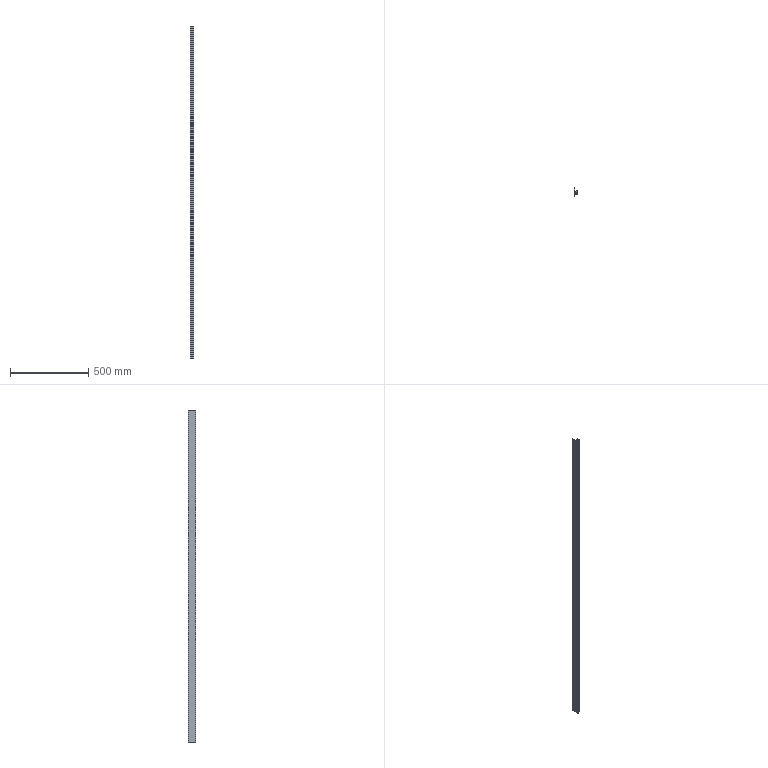Part | SolidWorks | features Extrusion 1 | 1 solid | 43 faces | box 25 x 50 x 2116 mm | volume 659198 mm3 | plane 35 | cylinder 8 | commonest cylinder face diameters 0.6 x8
STEP:
#1=CARTESIAN_POINT('',(1.5,0.,1058.));
#2=VERTEX_POINT('',#1);
#3=CARTESIAN_POINT('',(1.5,10.,1058.));
#4=VERTEX_POINT('',#3);
#5=CARTESIAN_POINT('',(1.5,0.,1058.));
#6=DIRECTION('',(0.,1.,0.));
#7=VECTOR('',#6,1000.);
#8=LINE('',#5,#7);
#9=EDGE_CURVE('',#2,#4,#8,.T.);
#10=ORIENTED_EDGE('',*,*,#9,.T.);
#11=CARTESIAN_POINT('',(4.,10.,1058.));
#12=VERTEX_POINT('',#11);
#13=CARTESIAN_POINT('',(1.5,10.,1058.));
#14=DIRECTION('',(1.,0.,0.));
#15=VECTOR('',#14,1000.);
#16=LINE('',#13,#15);
#17=EDGE_CURVE('',#4,#12,#16,.T.);
#18=ORIENTED_EDGE('',*,*,#17,.T.);
#19=CARTESIAN_POINT('',(4.,10.5,1058.));
#20=VERTEX_POINT('',#19);
#21=CARTESIAN_POINT('',(4.,10.,1058.));
#22=DIRECTION('',(0.,1.,0.));
#23=VECTOR('',#22,1000.);
#24=LINE('',#21,#23);
#25=EDGE_CURVE('',#12,#20,#24,.T.);
#26=ORIENTED_EDGE('',*,*,#25,.T.);
#27=CARTESIAN_POINT('',(8.9,10.5,1058.));
#28=VERTEX_POINT('',#27);
#29=CARTESIAN_POINT('',(4.,10.5,1058.));
#30=DIRECTION('',(1.,0.,0.));
#31=VECTOR('',#30,1000.);
#32=LINE('',#29,#31);
#33=EDGE_CURVE('',#20,#28,#32,.T.);
#34=ORIENTED_EDGE('',*,*,#33,.T.);
#35=CARTESIAN_POINT('',(8.9,12.2,1058.));
#36=VERTEX_POINT('',#35);
#37=CARTESIAN_POINT('',(8.9,10.5,1058.));
#38=DIRECTION('',(0.,1.,0.));
#39=VECTOR('',#38,1000.);
#40=LINE('',#37,#39);
#41=EDGE_CURVE('',#28,#36,#40,.T.);
#42=ORIENTED_EDGE('',*,*,#41,.T.);
#43=CARTESIAN_POINT('',(8.6,12.5,1058.));
#44=VERTEX_POINT('',#43);
#45=CARTESIAN_POINT('',(8.6,12.2,1058.));
#46=DIRECTION('',(0.,0.,1.));
#47=DIRECTION('',(1.,0.,0.));
#48=AXIS2_PLACEMENT_3D('',#45,#46,#47);
#49=CIRCLE('',#48,0.3);
#50=EDGE_CURVE('',#36,#44,#49,.T.);
#51=ORIENTED_EDGE('',*,*,#50,.T.);
#52=CARTESIAN_POINT('',(5.05,12.5,1058.));
#53=VERTEX_POINT('',#52);
#54=CARTESIAN_POINT('',(8.6,12.5,1058.));
#55=DIRECTION('',(-1.,0.,0.));
#56=VECTOR('',#55,1000.);
#57=LINE('',#54,#56);
#58=EDGE_CURVE('',#44,#53,#57,.T.);
#59=ORIENTED_EDGE('',*,*,#58,.T.);
#60=CARTESIAN_POINT('',(4.75,12.8,1058.));
#61=VERTEX_POINT('',#60);
#62=CARTESIAN_POINT('',(5.05,12.8,1058.));
#63=DIRECTION('',(0.,0.,-1.));
#64=DIRECTION('',(1.,0.,0.));
#65=AXIS2_PLACEMENT_3D('',#62,#63,#64);
#66=CIRCLE('',#65,0.3);
#67=EDGE_CURVE('',#53,#61,#66,.T.);
#68=ORIENTED_EDGE('',*,*,#67,.T.);
#69=CARTESIAN_POINT('',(4.75,16.153,1058.));
#70=VERTEX_POINT('',#69);
#71=CARTESIAN_POINT('',(4.75,12.8,1058.));
#72=DIRECTION('',(0.,1.,0.));
#73=VECTOR('',#72,1000.);
#74=LINE('',#71,#73);
#75=EDGE_CURVE('',#61,#70,#74,.T.);
#76=ORIENTED_EDGE('',*,*,#75,.T.);
#77=CARTESIAN_POINT('',(4.838,16.365,1058.));
#78=VERTEX_POINT('',#77);
#79=CARTESIAN_POINT('',(5.05,16.153,1058.));
#80=DIRECTION('',(0.,0.,-1.));
#81=DIRECTION('',(1.,0.,0.));
#82=AXIS2_PLACEMENT_3D('',#79,#80,#81);
#83=CIRCLE('',#82,0.3);
#84=EDGE_CURVE('',#70,#78,#83,.T.);
#85=ORIENTED_EDGE('',*,*,#84,.T.);
#86=CARTESIAN_POINT('',(8.785,20.312,1058.));
#87=VERTEX_POINT('',#86);
#88=CARTESIAN_POINT('',(4.838,16.365,1058.));
#89=DIRECTION('',(0.7071,0.7071,0.));
#90=VECTOR('',#89,1000.);
#91=LINE('',#88,#90);
#92=EDGE_CURVE('',#78,#87,#91,.T.);
#93=ORIENTED_EDGE('',*,*,#92,.T.);
#94=CARTESIAN_POINT('',(8.997,20.4,1058.));
#95=VERTEX_POINT('',#94);
#96=CARTESIAN_POINT('',(8.997,20.1,1058.));
#97=DIRECTION('',(0.,0.,-1.));
#98=DIRECTION('',(1.,0.,0.));
#99=AXIS2_PLACEMENT_3D('',#96,#97,#98);
#100=CIRCLE('',#99,0.3);
#101=EDGE_CURVE('',#87,#95,#100,.T.);
#102=ORIENTED_EDGE('',*,*,#101,.T.);
#103=CARTESIAN_POINT('',(17.003,20.4,1058.));
#104=VERTEX_POINT('',#103);
#105=CARTESIAN_POINT('',(8.997,20.4,1058.));
#106=DIRECTION('',(1.,0.,0.));
#107=VECTOR('',#106,1000.);
#108=LINE('',#105,#107);
#109=EDGE_CURVE('',#95,#104,#108,.T.);
#110=ORIENTED_EDGE('',*,*,#109,.T.);
#111=CARTESIAN_POINT('',(17.215,20.312,1058.));
#112=VERTEX_POINT('',#111);
#113=CARTESIAN_POINT('',(17.003,20.1,1058.));
#114=DIRECTION('',(0.,0.,-1.));
#115=DIRECTION('',(1.,0.,0.));
#116=AXIS2_PLACEMENT_3D('',#113,#114,#115);
#117=CIRCLE('',#116,0.3);
#118=EDGE_CURVE('',#104,#112,#117,.T.);
#119=ORIENTED_EDGE('',*,*,#118,.T.);
#120=CARTESIAN_POINT('',(21.162,16.365,1058.));
#121=VERTEX_POINT('',#120);
#122=CARTESIAN_POINT('',(17.215,20.312,1058.));
#123=DIRECTION('',(0.7071,-0.7071,0.));
#124=VECTOR('',#123,1000.);
#125=LINE('',#122,#124);
#126=EDGE_CURVE('',#112,#121,#125,.T.);
#127=ORIENTED_EDGE('',*,*,#126,.T.);
#128=CARTESIAN_POINT('',(21.25,16.153,1058.));
#129=VERTEX_POINT('',#128);
#130=CARTESIAN_POINT('',(20.95,16.153,1058.));
#131=DIRECTION('',(0.,0.,-1.));
#132=DIRECTION('',(1.,0.,0.));
#133=AXIS2_PLACEMENT_3D('',#130,#131,#132);
#134=CIRCLE('',#133,0.3);
#135=EDGE_CURVE('',#121,#129,#134,.T.);
#136=ORIENTED_EDGE('',*,*,#135,.T.);
#137=CARTESIAN_POINT('',(21.25,12.8,1058.));
#138=VERTEX_POINT('',#137);
#139=CARTESIAN_POINT('',(21.25,16.153,1058.));
#140=DIRECTION('',(0.,-1.,0.));
#141=VECTOR('',#140,1000.);
#142=LINE('',#139,#141);
#143=EDGE_CURVE('',#129,#138,#142,.T.);
#144=ORIENTED_EDGE('',*,*,#143,.T.);
#145=CARTESIAN_POINT('',(20.95,12.5,1058.));
#146=VERTEX_POINT('',#145);
#147=CARTESIAN_POINT('',(20.95,12.8,1058.));
#148=DIRECTION('',(0.,0.,-1.));
#149=DIRECTION('',(1.,0.,0.));
#150=AXIS2_PLACEMENT_3D('',#147,#148,#149);
#151=CIRCLE('',#150,0.3);
#152=EDGE_CURVE('',#138,#146,#151,.T.);
#153=ORIENTED_EDGE('',*,*,#152,.T.);
#154=CARTESIAN_POINT('',(17.4,12.5,1058.));
#155=VERTEX_POINT('',#154);
#156=CARTESIAN_POINT('',(20.95,12.5,1058.));
#157=DIRECTION('',(-1.,0.,0.));
#158=VECTOR('',#157,1000.);
#159=LINE('',#156,#158);
#160=EDGE_CURVE('',#146,#155,#159,.T.);
#161=ORIENTED_EDGE('',*,*,#160,.T.);
#162=CARTESIAN_POINT('',(17.1,12.2,1058.));
#163=VERTEX_POINT('',#162);
#164=CARTESIAN_POINT('',(17.4,12.2,1058.));
#165=DIRECTION('',(0.,0.,1.));
#166=DIRECTION('',(1.,0.,0.));
#167=AXIS2_PLACEMENT_3D('',#164,#165,#166);
#168=CIRCLE('',#167,0.3);
#169=EDGE_CURVE('',#155,#163,#168,.T.);
#170=ORIENTED_EDGE('',*,*,#169,.T.);
#171=CARTESIAN_POINT('',(17.1,10.5,1058.));
#172=VERTEX_POINT('',#171);
#173=CARTESIAN_POINT('',(17.1,12.2,1058.));
#174=DIRECTION('',(0.,-1.,0.));
#175=VECTOR('',#174,1000.);
#176=LINE('',#173,#175);
#177=EDGE_CURVE('',#163,#172,#176,.T.);
#178=ORIENTED_EDGE('',*,*,#177,.T.);
#179=CARTESIAN_POINT('',(22.,10.5,1058.));
#180=VERTEX_POINT('',#179);
#181=CARTESIAN_POINT('',(17.1,10.5,1058.));
#182=DIRECTION('',(1.,0.,0.));
#183=VECTOR('',#182,1000.);
#184=LINE('',#181,#183);
#185=EDGE_CURVE('',#172,#180,#184,.T.);
#186=ORIENTED_EDGE('',*,*,#185,.T.);
#187=CARTESIAN_POINT('',(22.,10.,1058.));
#188=VERTEX_POINT('',#187);
#189=CARTESIAN_POINT('',(22.,10.5,1058.));
#190=DIRECTION('',(0.,-1.,0.));
#191=VECTOR('',#190,1000.);
#192=LINE('',#189,#191);
#193=EDGE_CURVE('',#180,#188,#192,.T.);
#194=ORIENTED_EDGE('',*,*,#193,.T.);
#195=CARTESIAN_POINT('',(25.,10.,1058.));
#196=VERTEX_POINT('',#195);
#197=CARTESIAN_POINT('',(22.,10.,1058.));
#198=DIRECTION('',(1.,0.,0.));
#199=VECTOR('',#198,1000.);
#200=LINE('',#197,#199);
#201=EDGE_CURVE('',#188,#196,#200,.T.);
#202=ORIENTED_EDGE('',*,*,#201,.T.);
#203=CARTESIAN_POINT('',(25.,15.,1058.));
#204=VERTEX_POINT('',#203);
#205=CARTESIAN_POINT('',(25.,10.,1058.));
#206=DIRECTION('',(0.,1.,0.));
#207=VECTOR('',#206,1000.);
#208=LINE('',#205,#207);
#209=EDGE_CURVE('',#196,#204,#208,.T.);
#210=ORIENTED_EDGE('',*,*,#209,.T.);
#211=CARTESIAN_POINT('',(23.,15.,1058.));
#212=VERTEX_POINT('',#211);
#213=CARTESIAN_POINT('',(25.,15.,1058.));
#214=DIRECTION('',(-1.,0.,0.));
#215=VECTOR('',#214,1000.);
#216=LINE('',#213,#215);
#217=EDGE_CURVE('',#204,#212,#216,.T.);
#218=ORIENTED_EDGE('',*,*,#217,.T.);
#219=CARTESIAN_POINT('',(23.,29.246,1058.));
#220=VERTEX_POINT('',#219);
#221=CARTESIAN_POINT('',(23.,15.,1058.));
#222=DIRECTION('',(0.,1.,0.));
#223=VECTOR('',#222,1000.);
#224=LINE('',#221,#223);
#225=EDGE_CURVE('',#212,#220,#224,.T.);
#226=ORIENTED_EDGE('',*,*,#225,.T.);
#227=CARTESIAN_POINT('',(22.25,29.996,1058.));
#228=VERTEX_POINT('',#227);
#229=CARTESIAN_POINT('',(23.,29.246,1058.));
#230=DIRECTION('',(-0.7071,0.7071,0.));
#231=VECTOR('',#230,1000.);
#232=LINE('',#229,#231);
#233=EDGE_CURVE('',#220,#228,#232,.T.);
#234=ORIENTED_EDGE('',*,*,#233,.T.);
#235=CARTESIAN_POINT('',(4.,30.,1058.));
#236=VERTEX_POINT('',#235);
#237=CARTESIAN_POINT('',(22.25,29.996,1058.));
#238=DIRECTION('',(-1.,0.0002341,0.));
#239=VECTOR('',#238,1000.);
#240=LINE('',#237,#239);
#241=EDGE_CURVE('',#228,#236,#240,.T.);
#242=ORIENTED_EDGE('',*,*,#241,.T.);
#243=CARTESIAN_POINT('',(4.,34.998,1058.));
#244=VERTEX_POINT('',#243);
#245=CARTESIAN_POINT('',(4.,30.,1058.));
#246=DIRECTION('',(0.,1.,0.));
#247=VECTOR('',#246,1000.);
#248=LINE('',#245,#247);
#249=EDGE_CURVE('',#236,#244,#248,.T.);
#250=ORIENTED_EDGE('',*,*,#249,.T.);
#251=CARTESIAN_POINT('',(3.,34.998,1058.));
#252=VERTEX_POINT('',#251);
#253=CARTESIAN_POINT('',(4.,34.998,1058.));
#254=DIRECTION('',(-1.,0.,0.));
#255=VECTOR('',#254,1000.);
#256=LINE('',#253,#255);
#257=EDGE_CURVE('',#244,#252,#256,.T.);
#258=ORIENTED_EDGE('',*,*,#257,.T.);
#259=CARTESIAN_POINT('',(3.,43.,1058.));
#260=VERTEX_POINT('',#259);
#261=CARTESIAN_POINT('',(3.,34.998,1058.));
#262=DIRECTION('',(0.,1.,0.));
#263=VECTOR('',#262,1000.);
#264=LINE('',#261,#263);
#265=EDGE_CURVE('',#252,#260,#264,.T.);
#266=ORIENTED_EDGE('',*,*,#265,.T.);
#267=CARTESIAN_POINT('',(4.,43.,1058.));
#268=VERTEX_POINT('',#267);
#269=CARTESIAN_POINT('',(3.,43.,1058.));
#270=DIRECTION('',(1.,0.,0.));
#271=VECTOR('',#270,1000.);
#272=LINE('',#269,#271);
#273=EDGE_CURVE('',#260,#268,#272,.T.);
#274=ORIENTED_EDGE('',*,*,#273,.T.);
#275=CARTESIAN_POINT('',(4.,50.,1058.));
#276=VERTEX_POINT('',#275);
#277=CARTESIAN_POINT('',(4.,43.,1058.));
#278=DIRECTION('',(0.,1.,0.));
#279=VECTOR('',#278,1000.);
#280=LINE('',#277,#279);
#281=EDGE_CURVE('',#268,#276,#280,.T.);
#282=ORIENTED_EDGE('',*,*,#281,.T.);
#283=CARTESIAN_POINT('',(0.,50.,1058.));
#284=VERTEX_POINT('',#283);
#285=CARTESIAN_POINT('',(4.,50.,1058.));
#286=DIRECTION('',(-1.,0.,0.));
#287=VECTOR('',#286,1000.);
#288=LINE('',#285,#287);
#289=EDGE_CURVE('',#276,#284,#288,.T.);
#290=ORIENTED_EDGE('',*,*,#289,.T.);
#291=CARTESIAN_POINT('',(0.,0.,1058.));
#292=VERTEX_POINT('',#291);
#293=CARTESIAN_POINT('',(0.,50.,1058.));
#294=DIRECTION('',(0.,-1.,0.));
#295=VECTOR('',#294,1000.);
#296=LINE('',#293,#295);
#297=EDGE_CURVE('',#284,#292,#296,.T.);
#298=ORIENTED_EDGE('',*,*,#297,.T.);
#299=CARTESIAN_POINT('',(0.,0.,1058.));
#300=DIRECTION('',(1.,0.,0.));
#301=VECTOR('',#300,1000.);
#302=LINE('',#299,#301);
#303=EDGE_CURVE('',#292,#2,#302,.T.);
#304=ORIENTED_EDGE('',*,*,#303,.T.);
#305=EDGE_LOOP('',(#10,#18,#26,#34,#42,#51,#59,#68,#76,#85,#93,#102,#110,#119,#127,#136,#144,#153,#161,#170,#178,#186,#194,#202,#210,#218,#226,#234,#242,#250,#258,#266,#274,#282,#290,#298,#304));
#306=FACE_OUTER_BOUND('',#305,.T.);
#307=CARTESIAN_POINT('',(21.,28.,1058.));
#308=VERTEX_POINT('',#307);
#309=CARTESIAN_POINT('',(2.,28.,1058.));
#310=VERTEX_POINT('',#309);
#311=CARTESIAN_POINT('',(2.,28.,1058.));
#312=DIRECTION('',(-1.,0.,0.));
#313=VECTOR('',#312,1000.);
#314=LINE('',#311,#313);
#315=EDGE_CURVE('',#308,#310,#314,.T.);
#316=ORIENTED_EDGE('',*,*,#315,.F.);
#317=CARTESIAN_POINT('',(21.,22.4,1058.));
#318=VERTEX_POINT('',#317);
#319=CARTESIAN_POINT('',(21.,28.,1058.));
#320=DIRECTION('',(0.,1.,0.));
#321=VECTOR('',#320,1000.);
#322=LINE('',#319,#321);
#323=EDGE_CURVE('',#318,#308,#322,.T.);
#324=ORIENTED_EDGE('',*,*,#323,.F.);
#325=CARTESIAN_POINT('',(2.,22.4,1058.));
#326=VERTEX_POINT('',#325);
#327=CARTESIAN_POINT('',(21.,22.4,1058.));
#328=DIRECTION('',(1.,0.,0.));
#329=VECTOR('',#328,1000.);
#330=LINE('',#327,#329);
#331=EDGE_CURVE('',#326,#318,#330,.T.);
#332=ORIENTED_EDGE('',*,*,#331,.F.);
#333=CARTESIAN_POINT('',(2.,22.4,1058.));
#334=DIRECTION('',(0.,-1.,0.));
#335=VECTOR('',#334,1000.);
#336=LINE('',#333,#335);
#337=EDGE_CURVE('',#310,#326,#336,.T.);
#338=ORIENTED_EDGE('',*,*,#337,.F.);
#339=EDGE_LOOP('',(#316,#324,#332,#338));
#340=FACE_BOUND('',#339,.T.);
#341=CARTESIAN_POINT('',(8.6,12.2,1058.));
#342=DIRECTION('',(0.,0.,1.));
#343=DIRECTION('',(1.,0.,0.));
#344=AXIS2_PLACEMENT_3D('',#341,#342,#343);
#345=PLANE('',#344);
#346=ADVANCED_FACE('',(#306,#340),#345,.T.);
#347=CARTESIAN_POINT('',(1.5,0.,-1058.));
#348=VERTEX_POINT('',#347);
#349=CARTESIAN_POINT('',(1.5,10.,-1058.));
#350=VERTEX_POINT('',#349);
#351=CARTESIAN_POINT('',(1.5,0.,-1058.));
#352=DIRECTION('',(0.,1.,0.));
#353=VECTOR('',#352,1000.);
#354=LINE('',#351,#353);
#355=EDGE_CURVE('',#348,#350,#354,.T.);
#356=ORIENTED_EDGE('',*,*,#355,.F.);
#357=CARTESIAN_POINT('',(0.,0.,-1058.));
#358=VERTEX_POINT('',#357);
#359=CARTESIAN_POINT('',(0.,0.,-1058.));
#360=DIRECTION('',(1.,0.,0.));
#361=VECTOR('',#360,1000.);
#362=LINE('',#359,#361);
#363=EDGE_CURVE('',#358,#348,#362,.T.);
#364=ORIENTED_EDGE('',*,*,#363,.F.);
#365=CARTESIAN_POINT('',(0.,50.,-1058.));
#366=VERTEX_POINT('',#365);
#367=CARTESIAN_POINT('',(0.,50.,-1058.));
#368=DIRECTION('',(0.,-1.,0.));
#369=VECTOR('',#368,1000.);
#370=LINE('',#367,#369);
#371=EDGE_CURVE('',#366,#358,#370,.T.);
#372=ORIENTED_EDGE('',*,*,#371,.F.);
#373=CARTESIAN_POINT('',(4.,50.,-1058.));
#374=VERTEX_POINT('',#373);
#375=CARTESIAN_POINT('',(4.,50.,-1058.));
#376=DIRECTION('',(-1.,0.,0.));
#377=VECTOR('',#376,1000.);
#378=LINE('',#375,#377);
#379=EDGE_CURVE('',#374,#366,#378,.T.);
#380=ORIENTED_EDGE('',*,*,#379,.F.);
#381=CARTESIAN_POINT('',(4.,43.,-1058.));
#382=VERTEX_POINT('',#381);
#383=CARTESIAN_POINT('',(4.,43.,-1058.));
#384=DIRECTION('',(0.,1.,0.));
#385=VECTOR('',#384,1000.);
#386=LINE('',#383,#385);
#387=EDGE_CURVE('',#382,#374,#386,.T.);
#388=ORIENTED_EDGE('',*,*,#387,.F.);
#389=CARTESIAN_POINT('',(3.,43.,-1058.));
#390=VERTEX_POINT('',#389);
#391=CARTESIAN_POINT('',(3.,43.,-1058.));
#392=DIRECTION('',(1.,0.,0.));
#393=VECTOR('',#392,1000.);
#394=LINE('',#391,#393);
#395=EDGE_CURVE('',#390,#382,#394,.T.);
#396=ORIENTED_EDGE('',*,*,#395,.F.);
#397=CARTESIAN_POINT('',(3.,34.998,-1058.));
#398=VERTEX_POINT('',#397);
#399=CARTESIAN_POINT('',(3.,34.998,-1058.));
#400=DIRECTION('',(0.,1.,0.));
#401=VECTOR('',#400,1000.);
#402=LINE('',#399,#401);
#403=EDGE_CURVE('',#398,#390,#402,.T.);
#404=ORIENTED_EDGE('',*,*,#403,.F.);
#405=CARTESIAN_POINT('',(4.,34.998,-1058.));
#406=VERTEX_POINT('',#405);
#407=CARTESIAN_POINT('',(4.,34.998,-1058.));
#408=DIRECTION('',(-1.,0.,0.));
#409=VECTOR('',#408,1000.);
#410=LINE('',#407,#409);
#411=EDGE_CURVE('',#406,#398,#410,.T.);
#412=ORIENTED_EDGE('',*,*,#411,.F.);
#413=CARTESIAN_POINT('',(4.,30.,-1058.));
#414=VERTEX_POINT('',#413);
#415=CARTESIAN_POINT('',(4.,30.,-1058.));
#416=DIRECTION('',(0.,1.,0.));
#417=VECTOR('',#416,1000.);
#418=LINE('',#415,#417);
#419=EDGE_CURVE('',#414,#406,#418,.T.);
#420=ORIENTED_EDGE('',*,*,#419,.F.);
#421=CARTESIAN_POINT('',(22.25,29.996,-1058.));
#422=VERTEX_POINT('',#421);
#423=CARTESIAN_POINT('',(22.25,29.996,-1058.));
#424=DIRECTION('',(-1.,0.0002341,0.));
#425=VECTOR('',#424,1000.);
#426=LINE('',#423,#425);
#427=EDGE_CURVE('',#422,#414,#426,.T.);
#428=ORIENTED_EDGE('',*,*,#427,.F.);
#429=CARTESIAN_POINT('',(23.,29.246,-1058.));
#430=VERTEX_POINT('',#429);
#431=CARTESIAN_POINT('',(23.,29.246,-1058.));
#432=DIRECTION('',(-0.7071,0.7071,0.));
#433=VECTOR('',#432,1000.);
#434=LINE('',#431,#433);
#435=EDGE_CURVE('',#430,#422,#434,.T.);
#436=ORIENTED_EDGE('',*,*,#435,.F.);
#437=CARTESIAN_POINT('',(23.,15.,-1058.));
#438=VERTEX_POINT('',#437);
#439=CARTESIAN_POINT('',(23.,15.,-1058.));
#440=DIRECTION('',(0.,1.,0.));
#441=VECTOR('',#440,1000.);
#442=LINE('',#439,#441);
#443=EDGE_CURVE('',#438,#430,#442,.T.);
#444=ORIENTED_EDGE('',*,*,#443,.F.);
#445=CARTESIAN_POINT('',(25.,15.,-1058.));
#446=VERTEX_POINT('',#445);
#447=CARTESIAN_POINT('',(25.,15.,-1058.));
#448=DIRECTION('',(-1.,0.,0.));
#449=VECTOR('',#448,1000.);
#450=LINE('',#447,#449);
#451=EDGE_CURVE('',#446,#438,#450,.T.);
#452=ORIENTED_EDGE('',*,*,#451,.F.);
#453=CARTESIAN_POINT('',(25.,10.,-1058.));
#454=VERTEX_POINT('',#453);
#455=CARTESIAN_POINT('',(25.,10.,-1058.));
#456=DIRECTION('',(0.,1.,0.));
#457=VECTOR('',#456,1000.);
#458=LINE('',#455,#457);
#459=EDGE_CURVE('',#454,#446,#458,.T.);
#460=ORIENTED_EDGE('',*,*,#459,.F.);
#461=CARTESIAN_POINT('',(22.,10.,-1058.));
#462=VERTEX_POINT('',#461);
#463=CARTESIAN_POINT('',(22.,10.,-1058.));
#464=DIRECTION('',(1.,0.,0.));
#465=VECTOR('',#464,1000.);
#466=LINE('',#463,#465);
#467=EDGE_CURVE('',#462,#454,#466,.T.);
#468=ORIENTED_EDGE('',*,*,#467,.F.);
#469=CARTESIAN_POINT('',(22.,10.5,-1058.));
#470=VERTEX_POINT('',#469);
#471=CARTESIAN_POINT('',(22.,10.5,-1058.));
#472=DIRECTION('',(0.,-1.,0.));
#473=VECTOR('',#472,1000.);
#474=LINE('',#471,#473);
#475=EDGE_CURVE('',#470,#462,#474,.T.);
#476=ORIENTED_EDGE('',*,*,#475,.F.);
#477=CARTESIAN_POINT('',(17.1,10.5,-1058.));
#478=VERTEX_POINT('',#477);
#479=CARTESIAN_POINT('',(17.1,10.5,-1058.));
#480=DIRECTION('',(1.,0.,0.));
#481=VECTOR('',#480,1000.);
#482=LINE('',#479,#481);
#483=EDGE_CURVE('',#478,#470,#482,.T.);
#484=ORIENTED_EDGE('',*,*,#483,.F.);
#485=CARTESIAN_POINT('',(17.1,12.2,-1058.));
#486=VERTEX_POINT('',#485);
#487=CARTESIAN_POINT('',(17.1,12.2,-1058.));
#488=DIRECTION('',(0.,-1.,0.));
#489=VECTOR('',#488,1000.);
#490=LINE('',#487,#489);
#491=EDGE_CURVE('',#486,#478,#490,.T.);
#492=ORIENTED_EDGE('',*,*,#491,.F.);
#493=CARTESIAN_POINT('',(17.4,12.5,-1058.));
#494=VERTEX_POINT('',#493);
#495=CARTESIAN_POINT('',(17.4,12.2,-1058.));
#496=DIRECTION('',(0.,0.,1.));
#497=DIRECTION('',(1.,0.,0.));
#498=AXIS2_PLACEMENT_3D('',#495,#496,#497);
#499=CIRCLE('',#498,0.3);
#500=EDGE_CURVE('',#494,#486,#499,.T.);
#501=ORIENTED_EDGE('',*,*,#500,.F.);
#502=CARTESIAN_POINT('',(20.95,12.5,-1058.));
#503=VERTEX_POINT('',#502);
#504=CARTESIAN_POINT('',(20.95,12.5,-1058.));
#505=DIRECTION('',(-1.,0.,0.));
#506=VECTOR('',#505,1000.);
#507=LINE('',#504,#506);
#508=EDGE_CURVE('',#503,#494,#507,.T.);
#509=ORIENTED_EDGE('',*,*,#508,.F.);
#510=CARTESIAN_POINT('',(21.25,12.8,-1058.));
#511=VERTEX_POINT('',#510);
#512=CARTESIAN_POINT('',(20.95,12.8,-1058.));
#513=DIRECTION('',(0.,0.,-1.));
#514=DIRECTION('',(1.,0.,0.));
#515=AXIS2_PLACEMENT_3D('',#512,#513,#514);
#516=CIRCLE('',#515,0.3);
#517=EDGE_CURVE('',#511,#503,#516,.T.);
#518=ORIENTED_EDGE('',*,*,#517,.F.);
#519=CARTESIAN_POINT('',(21.25,16.153,-1058.));
#520=VERTEX_POINT('',#519);
#521=CARTESIAN_POINT('',(21.25,16.153,-1058.));
#522=DIRECTION('',(0.,-1.,0.));
#523=VECTOR('',#522,1000.);
#524=LINE('',#521,#523);
#525=EDGE_CURVE('',#520,#511,#524,.T.);
#526=ORIENTED_EDGE('',*,*,#525,.F.);
#527=CARTESIAN_POINT('',(21.162,16.365,-1058.));
#528=VERTEX_POINT('',#527);
#529=CARTESIAN_POINT('',(20.95,16.153,-1058.));
#530=DIRECTION('',(0.,0.,-1.));
#531=DIRECTION('',(1.,0.,0.));
#532=AXIS2_PLACEMENT_3D('',#529,#530,#531);
#533=CIRCLE('',#532,0.3);
#534=EDGE_CURVE('',#528,#520,#533,.T.);
#535=ORIENTED_EDGE('',*,*,#534,.F.);
#536=CARTESIAN_POINT('',(17.215,20.312,-1058.));
#537=VERTEX_POINT('',#536);
#538=CARTESIAN_POINT('',(17.215,20.312,-1058.));
#539=DIRECTION('',(0.7071,-0.7071,0.));
#540=VECTOR('',#539,1000.);
#541=LINE('',#538,#540);
#542=EDGE_CURVE('',#537,#528,#541,.T.);
#543=ORIENTED_EDGE('',*,*,#542,.F.);
#544=CARTESIAN_POINT('',(17.003,20.4,-1058.));
#545=VERTEX_POINT('',#544);
#546=CARTESIAN_POINT('',(17.003,20.1,-1058.));
#547=DIRECTION('',(0.,0.,-1.));
#548=DIRECTION('',(1.,0.,0.));
#549=AXIS2_PLACEMENT_3D('',#546,#547,#548);
#550=CIRCLE('',#549,0.3);
#551=EDGE_CURVE('',#545,#537,#550,.T.);
#552=ORIENTED_EDGE('',*,*,#551,.F.);
#553=CARTESIAN_POINT('',(8.997,20.4,-1058.));
#554=VERTEX_POINT('',#553);
#555=CARTESIAN_POINT('',(8.997,20.4,-1058.));
#556=DIRECTION('',(1.,0.,0.));
#557=VECTOR('',#556,1000.);
#558=LINE('',#555,#557);
#559=EDGE_CURVE('',#554,#545,#558,.T.);
#560=ORIENTED_EDGE('',*,*,#559,.F.);
#561=CARTESIAN_POINT('',(8.785,20.312,-1058.));
#562=VERTEX_POINT('',#561);
#563=CARTESIAN_POINT('',(8.997,20.1,-1058.));
#564=DIRECTION('',(0.,0.,-1.));
#565=DIRECTION('',(1.,0.,0.));
#566=AXIS2_PLACEMENT_3D('',#563,#564,#565);
#567=CIRCLE('',#566,0.3);
#568=EDGE_CURVE('',#562,#554,#567,.T.);
#569=ORIENTED_EDGE('',*,*,#568,.F.);
#570=CARTESIAN_POINT('',(4.838,16.365,-1058.));
#571=VERTEX_POINT('',#570);
#572=CARTESIAN_POINT('',(4.838,16.365,-1058.));
#573=DIRECTION('',(0.7071,0.7071,0.));
#574=VECTOR('',#573,1000.);
#575=LINE('',#572,#574);
#576=EDGE_CURVE('',#571,#562,#575,.T.);
#577=ORIENTED_EDGE('',*,*,#576,.F.);
#578=CARTESIAN_POINT('',(4.75,16.153,-1058.));
#579=VERTEX_POINT('',#578);
#580=CARTESIAN_POINT('',(5.05,16.153,-1058.));
#581=DIRECTION('',(0.,0.,-1.));
#582=DIRECTION('',(1.,0.,0.));
#583=AXIS2_PLACEMENT_3D('',#580,#581,#582);
#584=CIRCLE('',#583,0.3);
#585=EDGE_CURVE('',#579,#571,#584,.T.);
#586=ORIENTED_EDGE('',*,*,#585,.F.);
#587=CARTESIAN_POINT('',(4.75,12.8,-1058.));
#588=VERTEX_POINT('',#587);
#589=CARTESIAN_POINT('',(4.75,12.8,-1058.));
#590=DIRECTION('',(0.,1.,0.));
#591=VECTOR('',#590,1000.);
#592=LINE('',#589,#591);
#593=EDGE_CURVE('',#588,#579,#592,.T.);
#594=ORIENTED_EDGE('',*,*,#593,.F.);
#595=CARTESIAN_POINT('',(5.05,12.5,-1058.));
#596=VERTEX_POINT('',#595);
#597=CARTESIAN_POINT('',(5.05,12.8,-1058.));
#598=DIRECTION('',(0.,0.,-1.));
#599=DIRECTION('',(1.,0.,0.));
#600=AXIS2_PLACEMENT_3D('',#597,#598,#599);
#601=CIRCLE('',#600,0.3);
#602=EDGE_CURVE('',#596,#588,#601,.T.);
#603=ORIENTED_EDGE('',*,*,#602,.F.);
#604=CARTESIAN_POINT('',(8.6,12.5,-1058.));
#605=VERTEX_POINT('',#604);
#606=CARTESIAN_POINT('',(8.6,12.5,-1058.));
#607=DIRECTION('',(-1.,0.,0.));
#608=VECTOR('',#607,1000.);
#609=LINE('',#606,#608);
#610=EDGE_CURVE('',#605,#596,#609,.T.);
#611=ORIENTED_EDGE('',*,*,#610,.F.);
#612=CARTESIAN_POINT('',(8.9,12.2,-1058.));
#613=VERTEX_POINT('',#612);
#614=CARTESIAN_POINT('',(8.6,12.2,-1058.));
#615=DIRECTION('',(0.,0.,1.));
#616=DIRECTION('',(1.,0.,0.));
#617=AXIS2_PLACEMENT_3D('',#614,#615,#616);
#618=CIRCLE('',#617,0.3);
#619=EDGE_CURVE('',#613,#605,#618,.T.);
#620=ORIENTED_EDGE('',*,*,#619,.F.);
#621=CARTESIAN_POINT('',(8.9,10.5,-1058.));
#622=VERTEX_POINT('',#621);
#623=CARTESIAN_POINT('',(8.9,10.5,-1058.));
#624=DIRECTION('',(0.,1.,0.));
#625=VECTOR('',#624,1000.);
#626=LINE('',#623,#625);
#627=EDGE_CURVE('',#622,#613,#626,.T.);
#628=ORIENTED_EDGE('',*,*,#627,.F.);
#629=CARTESIAN_POINT('',(4.,10.5,-1058.));
#630=VERTEX_POINT('',#629);
#631=CARTESIAN_POINT('',(4.,10.5,-1058.));
#632=DIRECTION('',(1.,0.,0.));
#633=VECTOR('',#632,1000.);
#634=LINE('',#631,#633);
#635=EDGE_CURVE('',#630,#622,#634,.T.);
#636=ORIENTED_EDGE('',*,*,#635,.F.);
#637=CARTESIAN_POINT('',(4.,10.,-1058.));
#638=VERTEX_POINT('',#637);
#639=CARTESIAN_POINT('',(4.,10.,-1058.));
#640=DIRECTION('',(0.,1.,0.));
#641=VECTOR('',#640,1000.);
#642=LINE('',#639,#641);
#643=EDGE_CURVE('',#638,#630,#642,.T.);
#644=ORIENTED_EDGE('',*,*,#643,.F.);
#645=CARTESIAN_POINT('',(1.5,10.,-1058.));
#646=DIRECTION('',(1.,0.,0.));
#647=VECTOR('',#646,1000.);
#648=LINE('',#645,#647);
#649=EDGE_CURVE('',#350,#638,#648,.T.);
#650=ORIENTED_EDGE('',*,*,#649,.F.);
#651=EDGE_LOOP('',(#356,#364,#372,#380,#388,#396,#404,#412,#420,#428,#436,#444,#452,#460,#468,#476,#484,#492,#501,#509,#518,#526,#535,#543,#552,#560,#569,#577,#586,#594,#603,#611,#620,#628,#636,#644,#650));
#652=FACE_OUTER_BOUND('',#651,.T.);
#653=CARTESIAN_POINT('',(21.,22.4,-1058.));
#654=VERTEX_POINT('',#653);
#655=CARTESIAN_POINT('',(21.,28.,-1058.));
#656=VERTEX_POINT('',#655);
#657=CARTESIAN_POINT('',(21.,28.,-1058.));
#658=DIRECTION('',(0.,1.,0.));
#659=VECTOR('',#658,1000.);
#660=LINE('',#657,#659);
#661=EDGE_CURVE('',#654,#656,#660,.T.);
#662=ORIENTED_EDGE('',*,*,#661,.T.);
#663=CARTESIAN_POINT('',(2.,28.,-1058.));
#664=VERTEX_POINT('',#663);
#665=CARTESIAN_POINT('',(2.,28.,-1058.));
#666=DIRECTION('',(-1.,0.,0.));
#667=VECTOR('',#666,1000.);
#668=LINE('',#665,#667);
#669=EDGE_CURVE('',#656,#664,#668,.T.);
#670=ORIENTED_EDGE('',*,*,#669,.T.);
#671=CARTESIAN_POINT('',(2.,22.4,-1058.));
#672=VERTEX_POINT('',#671);
#673=CARTESIAN_POINT('',(2.,22.4,-1058.));
#674=DIRECTION('',(0.,-1.,0.));
#675=VECTOR('',#674,1000.);
#676=LINE('',#673,#675);
#677=EDGE_CURVE('',#664,#672,#676,.T.);
#678=ORIENTED_EDGE('',*,*,#677,.T.);
#679=CARTESIAN_POINT('',(21.,22.4,-1058.));
#680=DIRECTION('',(1.,0.,0.));
#681=VECTOR('',#680,1000.);
#682=LINE('',#679,#681);
#683=EDGE_CURVE('',#672,#654,#682,.T.);
#684=ORIENTED_EDGE('',*,*,#683,.T.);
#685=EDGE_LOOP('',(#662,#670,#678,#684));
#686=FACE_BOUND('',#685,.T.);
#687=CARTESIAN_POINT('',(8.6,12.2,-1058.));
#688=DIRECTION('',(0.,0.,1.));
#689=DIRECTION('',(1.,0.,0.));
#690=AXIS2_PLACEMENT_3D('',#687,#688,#689);
#691=PLANE('',#690);
#692=ADVANCED_FACE('',(#652,#686),#691,.F.);
#693=ORIENTED_EDGE('',*,*,#355,.T.);
#694=CARTESIAN_POINT('',(1.5,10.,1058.));
#695=DIRECTION('',(0.,0.,-1.));
#696=VECTOR('',#695,1000.);
#697=LINE('',#694,#696);
#698=EDGE_CURVE('',#4,#350,#697,.T.);
#699=ORIENTED_EDGE('',*,*,#698,.F.);
#700=ORIENTED_EDGE('',*,*,#9,.F.);
#701=CARTESIAN_POINT('',(1.5,0.,1058.));
#702=DIRECTION('',(0.,0.,-1.));
#703=VECTOR('',#702,1000.);
#704=LINE('',#701,#703);
#705=EDGE_CURVE('',#2,#348,#704,.T.);
#706=ORIENTED_EDGE('',*,*,#705,.T.);
#707=EDGE_LOOP('',(#693,#699,#700,#706));
#708=FACE_OUTER_BOUND('',#707,.T.);
#709=CARTESIAN_POINT('',(1.5,0.,1058.));
#710=DIRECTION('',(-1.,0.,0.));
#711=DIRECTION('',(0.,0.,1.));
#712=AXIS2_PLACEMENT_3D('',#709,#710,#711);
#713=PLANE('',#712);
#714=ADVANCED_FACE('',(#708),#713,.F.);
#715=ORIENTED_EDGE('',*,*,#649,.T.);
#716=CARTESIAN_POINT('',(4.,10.,1058.));
#717=DIRECTION('',(0.,0.,-1.));
#718=VECTOR('',#717,1000.);
#719=LINE('',#716,#718);
#720=EDGE_CURVE('',#12,#638,#719,.T.);
#721=ORIENTED_EDGE('',*,*,#720,.F.);
#722=ORIENTED_EDGE('',*,*,#17,.F.);
#723=ORIENTED_EDGE('',*,*,#698,.T.);
#724=EDGE_LOOP('',(#715,#721,#722,#723));
#725=FACE_OUTER_BOUND('',#724,.T.);
#726=CARTESIAN_POINT('',(1.5,10.,1058.));
#727=DIRECTION('',(0.,1.,0.));
#728=DIRECTION('',(0.,0.,1.));
#729=AXIS2_PLACEMENT_3D('',#726,#727,#728);
#730=PLANE('',#729);
#731=ADVANCED_FACE('',(#725),#730,.F.);
#732=ORIENTED_EDGE('',*,*,#643,.T.);
#733=CARTESIAN_POINT('',(4.,10.5,1058.));
#734=DIRECTION('',(0.,0.,-1.));
#735=VECTOR('',#734,1000.);
#736=LINE('',#733,#735);
#737=EDGE_CURVE('',#20,#630,#736,.T.);
#738=ORIENTED_EDGE('',*,*,#737,.F.);
#739=ORIENTED_EDGE('',*,*,#25,.F.);
#740=ORIENTED_EDGE('',*,*,#720,.T.);
#741=EDGE_LOOP('',(#732,#738,#739,#740));
#742=FACE_OUTER_BOUND('',#741,.T.);
#743=CARTESIAN_POINT('',(4.,10.,1058.));
#744=DIRECTION('',(-1.,0.,0.));
#745=DIRECTION('',(0.,0.,1.));
#746=AXIS2_PLACEMENT_3D('',#743,#744,#745);
#747=PLANE('',#746);
#748=ADVANCED_FACE('',(#742),#747,.F.);
#749=ORIENTED_EDGE('',*,*,#635,.T.);
#750=CARTESIAN_POINT('',(8.9,10.5,1058.));
#751=DIRECTION('',(0.,0.,-1.));
#752=VECTOR('',#751,1000.);
#753=LINE('',#750,#752);
#754=EDGE_CURVE('',#28,#622,#753,.T.);
#755=ORIENTED_EDGE('',*,*,#754,.F.);
#756=ORIENTED_EDGE('',*,*,#33,.F.);
#757=ORIENTED_EDGE('',*,*,#737,.T.);
#758=EDGE_LOOP('',(#749,#755,#756,#757));
#759=FACE_OUTER_BOUND('',#758,.T.);
#760=CARTESIAN_POINT('',(4.,10.5,1058.));
#761=DIRECTION('',(0.,1.,0.));
#762=DIRECTION('',(0.,0.,1.));
#763=AXIS2_PLACEMENT_3D('',#760,#761,#762);
#764=PLANE('',#763);
#765=ADVANCED_FACE('',(#759),#764,.F.);
#766=ORIENTED_EDGE('',*,*,#627,.T.);
#767=CARTESIAN_POINT('',(8.9,12.2,1058.));
#768=DIRECTION('',(0.,0.,-1.));
#769=VECTOR('',#768,1000.);
#770=LINE('',#767,#769);
#771=EDGE_CURVE('',#36,#613,#770,.T.);
#772=ORIENTED_EDGE('',*,*,#771,.F.);
#773=ORIENTED_EDGE('',*,*,#41,.F.);
#774=ORIENTED_EDGE('',*,*,#754,.T.);
#775=EDGE_LOOP('',(#766,#772,#773,#774));
#776=FACE_OUTER_BOUND('',#775,.T.);
#777=CARTESIAN_POINT('',(8.9,10.5,1058.));
#778=DIRECTION('',(-1.,0.,0.));
#779=DIRECTION('',(0.,0.,1.));
#780=AXIS2_PLACEMENT_3D('',#777,#778,#779);
#781=PLANE('',#780);
#782=ADVANCED_FACE('',(#776),#781,.F.);
#783=ORIENTED_EDGE('',*,*,#619,.T.);
#784=CARTESIAN_POINT('',(8.6,12.5,1058.));
#785=DIRECTION('',(0.,0.,-1.));
#786=VECTOR('',#785,1000.);
#787=LINE('',#784,#786);
#788=EDGE_CURVE('',#44,#605,#787,.T.);
#789=ORIENTED_EDGE('',*,*,#788,.F.);
#790=ORIENTED_EDGE('',*,*,#50,.F.);
#791=ORIENTED_EDGE('',*,*,#771,.T.);
#792=EDGE_LOOP('',(#783,#789,#790,#791));
#793=FACE_OUTER_BOUND('',#792,.T.);
#794=CARTESIAN_POINT('',(8.6,12.2,1058.));
#795=DIRECTION('',(0.,0.,-1.));
#796=DIRECTION('',(-1.,0.,0.));
#797=AXIS2_PLACEMENT_3D('',#794,#795,#796);
#798=CYLINDRICAL_SURFACE('',#797,0.3);
#799=ADVANCED_FACE('',(#793),#798,.T.);
#800=ORIENTED_EDGE('',*,*,#610,.T.);
#801=CARTESIAN_POINT('',(5.05,12.5,1058.));
#802=DIRECTION('',(0.,0.,-1.));
#803=VECTOR('',#802,1000.);
#804=LINE('',#801,#803);
#805=EDGE_CURVE('',#53,#596,#804,.T.);
#806=ORIENTED_EDGE('',*,*,#805,.F.);
#807=ORIENTED_EDGE('',*,*,#58,.F.);
#808=ORIENTED_EDGE('',*,*,#788,.T.);
#809=EDGE_LOOP('',(#800,#806,#807,#808));
#810=FACE_OUTER_BOUND('',#809,.T.);
#811=CARTESIAN_POINT('',(8.6,12.5,1058.));
#812=DIRECTION('',(0.,-1.,0.));
#813=DIRECTION('',(0.,0.,-1.));
#814=AXIS2_PLACEMENT_3D('',#811,#812,#813);
#815=PLANE('',#814);
#816=ADVANCED_FACE('',(#810),#815,.F.);
#817=ORIENTED_EDGE('',*,*,#602,.T.);
#818=CARTESIAN_POINT('',(4.75,12.8,1058.));
#819=DIRECTION('',(0.,0.,-1.));
#820=VECTOR('',#819,1000.);
#821=LINE('',#818,#820);
#822=EDGE_CURVE('',#61,#588,#821,.T.);
#823=ORIENTED_EDGE('',*,*,#822,.F.);
#824=ORIENTED_EDGE('',*,*,#67,.F.);
#825=ORIENTED_EDGE('',*,*,#805,.T.);
#826=EDGE_LOOP('',(#817,#823,#824,#825));
#827=FACE_OUTER_BOUND('',#826,.T.);
#828=CARTESIAN_POINT('',(5.05,12.8,1058.));
#829=DIRECTION('',(0.,0.,-1.));
#830=DIRECTION('',(-1.,0.,0.));
#831=AXIS2_PLACEMENT_3D('',#828,#829,#830);
#832=CYLINDRICAL_SURFACE('',#831,0.3);
#833=ADVANCED_FACE('',(#827),#832,.F.);
#834=ORIENTED_EDGE('',*,*,#593,.T.);
#835=CARTESIAN_POINT('',(4.75,16.153,1058.));
#836=DIRECTION('',(0.,0.,-1.));
#837=VECTOR('',#836,1000.);
#838=LINE('',#835,#837);
#839=EDGE_CURVE('',#70,#579,#838,.T.);
#840=ORIENTED_EDGE('',*,*,#839,.F.);
#841=ORIENTED_EDGE('',*,*,#75,.F.);
#842=ORIENTED_EDGE('',*,*,#822,.T.);
#843=EDGE_LOOP('',(#834,#840,#841,#842));
#844=FACE_OUTER_BOUND('',#843,.T.);
#845=CARTESIAN_POINT('',(4.75,12.8,1058.));
#846=DIRECTION('',(-1.,0.,0.));
#847=DIRECTION('',(0.,0.,1.));
#848=AXIS2_PLACEMENT_3D('',#845,#846,#847);
#849=PLANE('',#848);
#850=ADVANCED_FACE('',(#844),#849,.F.);
#851=ORIENTED_EDGE('',*,*,#585,.T.);
#852=CARTESIAN_POINT('',(4.838,16.365,1058.));
#853=DIRECTION('',(0.,0.,-1.));
#854=VECTOR('',#853,1000.);
#855=LINE('',#852,#854);
#856=EDGE_CURVE('',#78,#571,#855,.T.);
#857=ORIENTED_EDGE('',*,*,#856,.F.);
#858=ORIENTED_EDGE('',*,*,#84,.F.);
#859=ORIENTED_EDGE('',*,*,#839,.T.);
#860=EDGE_LOOP('',(#851,#857,#858,#859));
#861=FACE_OUTER_BOUND('',#860,.T.);
#862=CARTESIAN_POINT('',(5.05,16.153,1058.));
#863=DIRECTION('',(0.,0.,-1.));
#864=DIRECTION('',(-1.,0.,0.));
#865=AXIS2_PLACEMENT_3D('',#862,#863,#864);
#866=CYLINDRICAL_SURFACE('',#865,0.3);
#867=ADVANCED_FACE('',(#861),#866,.F.);
#868=ORIENTED_EDGE('',*,*,#576,.T.);
#869=CARTESIAN_POINT('',(8.785,20.312,1058.));
#870=DIRECTION('',(0.,0.,-1.));
#871=VECTOR('',#870,1000.);
#872=LINE('',#869,#871);
#873=EDGE_CURVE('',#87,#562,#872,.T.);
#874=ORIENTED_EDGE('',*,*,#873,.F.);
#875=ORIENTED_EDGE('',*,*,#92,.F.);
#876=ORIENTED_EDGE('',*,*,#856,.T.);
#877=EDGE_LOOP('',(#868,#874,#875,#876));
#878=FACE_OUTER_BOUND('',#877,.T.);
#879=CARTESIAN_POINT('',(4.838,16.365,1058.));
#880=DIRECTION('',(-0.7071,0.7071,0.));
#881=DIRECTION('',(-0.7071,-0.7071,0.));
#882=AXIS2_PLACEMENT_3D('',#879,#880,#881);
#883=PLANE('',#882);
#884=ADVANCED_FACE('',(#878),#883,.F.);
#885=ORIENTED_EDGE('',*,*,#568,.T.);
#886=CARTESIAN_POINT('',(8.997,20.4,1058.));
#887=DIRECTION('',(0.,0.,-1.));
#888=VECTOR('',#887,1000.);
#889=LINE('',#886,#888);
#890=EDGE_CURVE('',#95,#554,#889,.T.);
#891=ORIENTED_EDGE('',*,*,#890,.F.);
#892=ORIENTED_EDGE('',*,*,#101,.F.);
#893=ORIENTED_EDGE('',*,*,#873,.T.);
#894=EDGE_LOOP('',(#885,#891,#892,#893));
#895=FACE_OUTER_BOUND('',#894,.T.);
#896=CARTESIAN_POINT('',(8.997,20.1,1058.));
#897=DIRECTION('',(0.,0.,-1.));
#898=DIRECTION('',(-1.,0.,0.));
#899=AXIS2_PLACEMENT_3D('',#896,#897,#898);
#900=CYLINDRICAL_SURFACE('',#899,0.3);
#901=ADVANCED_FACE('',(#895),#900,.F.);
#902=ORIENTED_EDGE('',*,*,#559,.T.);
#903=CARTESIAN_POINT('',(17.003,20.4,1058.));
#904=DIRECTION('',(0.,0.,-1.));
#905=VECTOR('',#904,1000.);
#906=LINE('',#903,#905);
#907=EDGE_CURVE('',#104,#545,#906,.T.);
#908=ORIENTED_EDGE('',*,*,#907,.F.);
#909=ORIENTED_EDGE('',*,*,#109,.F.);
#910=ORIENTED_EDGE('',*,*,#890,.T.);
#911=EDGE_LOOP('',(#902,#908,#909,#910));
#912=FACE_OUTER_BOUND('',#911,.T.);
#913=CARTESIAN_POINT('',(8.997,20.4,1058.));
#914=DIRECTION('',(0.,1.,0.));
#915=DIRECTION('',(0.,0.,1.));
#916=AXIS2_PLACEMENT_3D('',#913,#914,#915);
#917=PLANE('',#916);
#918=ADVANCED_FACE('',(#912),#917,.F.);
#919=ORIENTED_EDGE('',*,*,#551,.T.);
#920=CARTESIAN_POINT('',(17.215,20.312,1058.));
#921=DIRECTION('',(0.,0.,-1.));
#922=VECTOR('',#921,1000.);
#923=LINE('',#920,#922);
#924=EDGE_CURVE('',#112,#537,#923,.T.);
#925=ORIENTED_EDGE('',*,*,#924,.F.);
#926=ORIENTED_EDGE('',*,*,#118,.F.);
#927=ORIENTED_EDGE('',*,*,#907,.T.);
#928=EDGE_LOOP('',(#919,#925,#926,#927));
#929=FACE_OUTER_BOUND('',#928,.T.);
#930=CARTESIAN_POINT('',(17.003,20.1,1058.));
#931=DIRECTION('',(0.,0.,-1.));
#932=DIRECTION('',(-1.,0.,0.));
#933=AXIS2_PLACEMENT_3D('',#930,#931,#932);
#934=CYLINDRICAL_SURFACE('',#933,0.3);
#935=ADVANCED_FACE('',(#929),#934,.F.);
#936=ORIENTED_EDGE('',*,*,#542,.T.);
#937=CARTESIAN_POINT('',(21.162,16.365,1058.));
#938=DIRECTION('',(0.,0.,-1.));
#939=VECTOR('',#938,1000.);
#940=LINE('',#937,#939);
#941=EDGE_CURVE('',#121,#528,#940,.T.);
#942=ORIENTED_EDGE('',*,*,#941,.F.);
#943=ORIENTED_EDGE('',*,*,#126,.F.);
#944=ORIENTED_EDGE('',*,*,#924,.T.);
#945=EDGE_LOOP('',(#936,#942,#943,#944));
#946=FACE_OUTER_BOUND('',#945,.T.);
#947=CARTESIAN_POINT('',(17.215,20.312,1058.));
#948=DIRECTION('',(0.7071,0.7071,0.));
#949=DIRECTION('',(-0.7071,0.7071,0.));
#950=AXIS2_PLACEMENT_3D('',#947,#948,#949);
#951=PLANE('',#950);
#952=ADVANCED_FACE('',(#946),#951,.F.);
#953=ORIENTED_EDGE('',*,*,#534,.T.);
#954=CARTESIAN_POINT('',(21.25,16.153,1058.));
#955=DIRECTION('',(0.,0.,-1.));
#956=VECTOR('',#955,1000.);
#957=LINE('',#954,#956);
#958=EDGE_CURVE('',#129,#520,#957,.T.);
#959=ORIENTED_EDGE('',*,*,#958,.F.);
#960=ORIENTED_EDGE('',*,*,#135,.F.);
#961=ORIENTED_EDGE('',*,*,#941,.T.);
#962=EDGE_LOOP('',(#953,#959,#960,#961));
#963=FACE_OUTER_BOUND('',#962,.T.);
#964=CARTESIAN_POINT('',(20.95,16.153,1058.));
#965=DIRECTION('',(0.,0.,-1.));
#966=DIRECTION('',(-1.,0.,0.));
#967=AXIS2_PLACEMENT_3D('',#964,#965,#966);
#968=CYLINDRICAL_SURFACE('',#967,0.3);
#969=ADVANCED_FACE('',(#963),#968,.F.);
#970=ORIENTED_EDGE('',*,*,#525,.T.);
#971=CARTESIAN_POINT('',(21.25,12.8,1058.));
#972=DIRECTION('',(0.,0.,-1.));
#973=VECTOR('',#972,1000.);
#974=LINE('',#971,#973);
#975=EDGE_CURVE('',#138,#511,#974,.T.);
#976=ORIENTED_EDGE('',*,*,#975,.F.);
#977=ORIENTED_EDGE('',*,*,#143,.F.);
#978=ORIENTED_EDGE('',*,*,#958,.T.);
#979=EDGE_LOOP('',(#970,#976,#977,#978));
#980=FACE_OUTER_BOUND('',#979,.T.);
#981=CARTESIAN_POINT('',(21.25,16.153,1058.));
#982=DIRECTION('',(1.,0.,0.));
#983=DIRECTION('',(0.,0.,-1.));
#984=AXIS2_PLACEMENT_3D('',#981,#982,#983);
#985=PLANE('',#984);
#986=ADVANCED_FACE('',(#980),#985,.F.);
#987=ORIENTED_EDGE('',*,*,#517,.T.);
#988=CARTESIAN_POINT('',(20.95,12.5,1058.));
#989=DIRECTION('',(0.,0.,-1.));
#990=VECTOR('',#989,1000.);
#991=LINE('',#988,#990);
#992=EDGE_CURVE('',#146,#503,#991,.T.);
#993=ORIENTED_EDGE('',*,*,#992,.F.);
#994=ORIENTED_EDGE('',*,*,#152,.F.);
#995=ORIENTED_EDGE('',*,*,#975,.T.);
#996=EDGE_LOOP('',(#987,#993,#994,#995));
#997=FACE_OUTER_BOUND('',#996,.T.);
#998=CARTESIAN_POINT('',(20.95,12.8,1058.));
#999=DIRECTION('',(0.,0.,-1.));
#1000=DIRECTION('',(-1.,0.,0.));
#1001=AXIS2_PLACEMENT_3D('',#998,#999,#1000);
#1002=CYLINDRICAL_SURFACE('',#1001,0.3);
#1003=ADVANCED_FACE('',(#997),#1002,.F.);
#1004=ORIENTED_EDGE('',*,*,#508,.T.);
#1005=CARTESIAN_POINT('',(17.4,12.5,1058.));
#1006=DIRECTION('',(0.,0.,-1.));
#1007=VECTOR('',#1006,1000.);
#1008=LINE('',#1005,#1007);
#1009=EDGE_CURVE('',#155,#494,#1008,.T.);
#1010=ORIENTED_EDGE('',*,*,#1009,.F.);
#1011=ORIENTED_EDGE('',*,*,#160,.F.);
#1012=ORIENTED_EDGE('',*,*,#992,.T.);
#1013=EDGE_LOOP('',(#1004,#1010,#1011,#1012));
#1014=FACE_OUTER_BOUND('',#1013,.T.);
#1015=CARTESIAN_POINT('',(20.95,12.5,1058.));
#1016=DIRECTION('',(0.,-1.,0.));
#1017=DIRECTION('',(0.,0.,-1.));
#1018=AXIS2_PLACEMENT_3D('',#1015,#1016,#1017);
#1019=PLANE('',#1018);
#1020=ADVANCED_FACE('',(#1014),#1019,.F.);
#1021=ORIENTED_EDGE('',*,*,#500,.T.);
#1022=CARTESIAN_POINT('',(17.1,12.2,1058.));
#1023=DIRECTION('',(0.,0.,-1.));
#1024=VECTOR('',#1023,1000.);
#1025=LINE('',#1022,#1024);
#1026=EDGE_CURVE('',#163,#486,#1025,.T.);
#1027=ORIENTED_EDGE('',*,*,#1026,.F.);
#1028=ORIENTED_EDGE('',*,*,#169,.F.);
#1029=ORIENTED_EDGE('',*,*,#1009,.T.);
#1030=EDGE_LOOP('',(#1021,#1027,#1028,#1029));
#1031=FACE_OUTER_BOUND('',#1030,.T.);
#1032=CARTESIAN_POINT('',(17.4,12.2,1058.));
#1033=DIRECTION('',(0.,0.,-1.));
#1034=DIRECTION('',(-1.,0.,0.));
#1035=AXIS2_PLACEMENT_3D('',#1032,#1033,#1034);
#1036=CYLINDRICAL_SURFACE('',#1035,0.3);
#1037=ADVANCED_FACE('',(#1031),#1036,.T.);
#1038=ORIENTED_EDGE('',*,*,#491,.T.);
#1039=CARTESIAN_POINT('',(17.1,10.5,1058.));
#1040=DIRECTION('',(0.,0.,-1.));
#1041=VECTOR('',#1040,1000.);
#1042=LINE('',#1039,#1041);
#1043=EDGE_CURVE('',#172,#478,#1042,.T.);
#1044=ORIENTED_EDGE('',*,*,#1043,.F.);
#1045=ORIENTED_EDGE('',*,*,#177,.F.);
#1046=ORIENTED_EDGE('',*,*,#1026,.T.);
#1047=EDGE_LOOP('',(#1038,#1044,#1045,#1046));
#1048=FACE_OUTER_BOUND('',#1047,.T.);
#1049=CARTESIAN_POINT('',(17.1,12.2,1058.));
#1050=DIRECTION('',(1.,0.,0.));
#1051=DIRECTION('',(0.,0.,-1.));
#1052=AXIS2_PLACEMENT_3D('',#1049,#1050,#1051);
#1053=PLANE('',#1052);
#1054=ADVANCED_FACE('',(#1048),#1053,.F.);
#1055=ORIENTED_EDGE('',*,*,#483,.T.);
#1056=CARTESIAN_POINT('',(22.,10.5,1058.));
#1057=DIRECTION('',(0.,0.,-1.));
#1058=VECTOR('',#1057,1000.);
#1059=LINE('',#1056,#1058);
#1060=EDGE_CURVE('',#180,#470,#1059,.T.);
#1061=ORIENTED_EDGE('',*,*,#1060,.F.);
#1062=ORIENTED_EDGE('',*,*,#185,.F.);
#1063=ORIENTED_EDGE('',*,*,#1043,.T.);
#1064=EDGE_LOOP('',(#1055,#1061,#1062,#1063));
#1065=FACE_OUTER_BOUND('',#1064,.T.);
#1066=CARTESIAN_POINT('',(17.1,10.5,1058.));
#1067=DIRECTION('',(0.,1.,0.));
#1068=DIRECTION('',(0.,0.,1.));
#1069=AXIS2_PLACEMENT_3D('',#1066,#1067,#1068);
#1070=PLANE('',#1069);
#1071=ADVANCED_FACE('',(#1065),#1070,.F.);
#1072=ORIENTED_EDGE('',*,*,#475,.T.);
#1073=CARTESIAN_POINT('',(22.,10.,1058.));
#1074=DIRECTION('',(0.,0.,-1.));
#1075=VECTOR('',#1074,1000.);
#1076=LINE('',#1073,#1075);
#1077=EDGE_CURVE('',#188,#462,#1076,.T.);
#1078=ORIENTED_EDGE('',*,*,#1077,.F.);
#1079=ORIENTED_EDGE('',*,*,#193,.F.);
#1080=ORIENTED_EDGE('',*,*,#1060,.T.);
#1081=EDGE_LOOP('',(#1072,#1078,#1079,#1080));
#1082=FACE_OUTER_BOUND('',#1081,.T.);
#1083=CARTESIAN_POINT('',(22.,10.5,1058.));
#1084=DIRECTION('',(1.,0.,0.));
#1085=DIRECTION('',(0.,0.,-1.));
#1086=AXIS2_PLACEMENT_3D('',#1083,#1084,#1085);
#1087=PLANE('',#1086);
#1088=ADVANCED_FACE('',(#1082),#1087,.F.);
#1089=ORIENTED_EDGE('',*,*,#467,.T.);
#1090=CARTESIAN_POINT('',(25.,10.,1058.));
#1091=DIRECTION('',(0.,0.,-1.));
#1092=VECTOR('',#1091,1000.);
#1093=LINE('',#1090,#1092);
#1094=EDGE_CURVE('',#196,#454,#1093,.T.);
#1095=ORIENTED_EDGE('',*,*,#1094,.F.);
#1096=ORIENTED_EDGE('',*,*,#201,.F.);
#1097=ORIENTED_EDGE('',*,*,#1077,.T.);
#1098=EDGE_LOOP('',(#1089,#1095,#1096,#1097));
#1099=FACE_OUTER_BOUND('',#1098,.T.);
#1100=CARTESIAN_POINT('',(22.,10.,1058.));
#1101=DIRECTION('',(0.,1.,0.));
#1102=DIRECTION('',(0.,0.,1.));
#1103=AXIS2_PLACEMENT_3D('',#1100,#1101,#1102);
#1104=PLANE('',#1103);
#1105=ADVANCED_FACE('',(#1099),#1104,.F.);
#1106=ORIENTED_EDGE('',*,*,#459,.T.);
#1107=CARTESIAN_POINT('',(25.,15.,1058.));
#1108=DIRECTION('',(0.,0.,-1.));
#1109=VECTOR('',#1108,1000.);
#1110=LINE('',#1107,#1109);
#1111=EDGE_CURVE('',#204,#446,#1110,.T.);
#1112=ORIENTED_EDGE('',*,*,#1111,.F.);
#1113=ORIENTED_EDGE('',*,*,#209,.F.);
#1114=ORIENTED_EDGE('',*,*,#1094,.T.);
#1115=EDGE_LOOP('',(#1106,#1112,#1113,#1114));
#1116=FACE_OUTER_BOUND('',#1115,.T.);
#1117=CARTESIAN_POINT('',(25.,10.,1058.));
#1118=DIRECTION('',(-1.,0.,0.));
#1119=DIRECTION('',(0.,0.,1.));
#1120=AXIS2_PLACEMENT_3D('',#1117,#1118,#1119);
#1121=PLANE('',#1120);
#1122=ADVANCED_FACE('',(#1116),#1121,.F.);
#1123=ORIENTED_EDGE('',*,*,#451,.T.);
#1124=CARTESIAN_POINT('',(23.,15.,1058.));
#1125=DIRECTION('',(0.,0.,-1.));
#1126=VECTOR('',#1125,1000.);
#1127=LINE('',#1124,#1126);
#1128=EDGE_CURVE('',#212,#438,#1127,.T.);
#1129=ORIENTED_EDGE('',*,*,#1128,.F.);
#1130=ORIENTED_EDGE('',*,*,#217,.F.);
#1131=ORIENTED_EDGE('',*,*,#1111,.T.);
#1132=EDGE_LOOP('',(#1123,#1129,#1130,#1131));
#1133=FACE_OUTER_BOUND('',#1132,.T.);
#1134=CARTESIAN_POINT('',(25.,15.,1058.));
#1135=DIRECTION('',(0.,-1.,0.));
#1136=DIRECTION('',(0.,0.,-1.));
#1137=AXIS2_PLACEMENT_3D('',#1134,#1135,#1136);
#1138=PLANE('',#1137);
#1139=ADVANCED_FACE('',(#1133),#1138,.F.);
#1140=ORIENTED_EDGE('',*,*,#443,.T.);
#1141=CARTESIAN_POINT('',(23.,29.246,1058.));
#1142=DIRECTION('',(0.,0.,-1.));
#1143=VECTOR('',#1142,1000.);
#1144=LINE('',#1141,#1143);
#1145=EDGE_CURVE('',#220,#430,#1144,.T.);
#1146=ORIENTED_EDGE('',*,*,#1145,.F.);
#1147=ORIENTED_EDGE('',*,*,#225,.F.);
#1148=ORIENTED_EDGE('',*,*,#1128,.T.);
#1149=EDGE_LOOP('',(#1140,#1146,#1147,#1148));
#1150=FACE_OUTER_BOUND('',#1149,.T.);
#1151=CARTESIAN_POINT('',(23.,15.,1058.));
#1152=DIRECTION('',(-1.,0.,0.));
#1153=DIRECTION('',(0.,0.,1.));
#1154=AXIS2_PLACEMENT_3D('',#1151,#1152,#1153);
#1155=PLANE('',#1154);
#1156=ADVANCED_FACE('',(#1150),#1155,.F.);
#1157=ORIENTED_EDGE('',*,*,#435,.T.);
#1158=CARTESIAN_POINT('',(22.25,29.996,1058.));
#1159=DIRECTION('',(0.,0.,-1.));
#1160=VECTOR('',#1159,1000.);
#1161=LINE('',#1158,#1160);
#1162=EDGE_CURVE('',#228,#422,#1161,.T.);
#1163=ORIENTED_EDGE('',*,*,#1162,.F.);
#1164=ORIENTED_EDGE('',*,*,#233,.F.);
#1165=ORIENTED_EDGE('',*,*,#1145,.T.);
#1166=EDGE_LOOP('',(#1157,#1163,#1164,#1165));
#1167=FACE_OUTER_BOUND('',#1166,.T.);
#1168=CARTESIAN_POINT('',(23.,29.246,1058.));
#1169=DIRECTION('',(-0.7071,-0.7071,0.));
#1170=DIRECTION('',(0.7071,-0.7071,0.));
#1171=AXIS2_PLACEMENT_3D('',#1168,#1169,#1170);
#1172=PLANE('',#1171);
#1173=ADVANCED_FACE('',(#1167),#1172,.F.);
#1174=ORIENTED_EDGE('',*,*,#427,.T.);
#1175=CARTESIAN_POINT('',(4.,30.,1058.));
#1176=DIRECTION('',(0.,0.,-1.));
#1177=VECTOR('',#1176,1000.);
#1178=LINE('',#1175,#1177);
#1179=EDGE_CURVE('',#236,#414,#1178,.T.);
#1180=ORIENTED_EDGE('',*,*,#1179,.F.);
#1181=ORIENTED_EDGE('',*,*,#241,.F.);
#1182=ORIENTED_EDGE('',*,*,#1162,.T.);
#1183=EDGE_LOOP('',(#1174,#1180,#1181,#1182));
#1184=FACE_OUTER_BOUND('',#1183,.T.);
#1185=CARTESIAN_POINT('',(22.25,29.996,1058.));
#1186=DIRECTION('',(-0.0002341,-1.,0.));
#1187=DIRECTION('',(1.,-0.0002341,0.));
#1188=AXIS2_PLACEMENT_3D('',#1185,#1186,#1187);
#1189=PLANE('',#1188);
#1190=ADVANCED_FACE('',(#1184),#1189,.F.);
#1191=ORIENTED_EDGE('',*,*,#419,.T.);
#1192=CARTESIAN_POINT('',(4.,34.998,1058.));
#1193=DIRECTION('',(0.,0.,-1.));
#1194=VECTOR('',#1193,1000.);
#1195=LINE('',#1192,#1194);
#1196=EDGE_CURVE('',#244,#406,#1195,.T.);
#1197=ORIENTED_EDGE('',*,*,#1196,.F.);
#1198=ORIENTED_EDGE('',*,*,#249,.F.);
#1199=ORIENTED_EDGE('',*,*,#1179,.T.);
#1200=EDGE_LOOP('',(#1191,#1197,#1198,#1199));
#1201=FACE_OUTER_BOUND('',#1200,.T.);
#1202=CARTESIAN_POINT('',(4.,30.,1058.));
#1203=DIRECTION('',(-1.,0.,0.));
#1204=DIRECTION('',(0.,-1.,0.));
#1205=AXIS2_PLACEMENT_3D('',#1202,#1203,#1204);
#1206=PLANE('',#1205);
#1207=ADVANCED_FACE('',(#1201),#1206,.F.);
#1208=ORIENTED_EDGE('',*,*,#411,.T.);
#1209=CARTESIAN_POINT('',(3.,34.998,1058.));
#1210=DIRECTION('',(0.,0.,-1.));
#1211=VECTOR('',#1210,1000.);
#1212=LINE('',#1209,#1211);
#1213=EDGE_CURVE('',#252,#398,#1212,.T.);
#1214=ORIENTED_EDGE('',*,*,#1213,.F.);
#1215=ORIENTED_EDGE('',*,*,#257,.F.);
#1216=ORIENTED_EDGE('',*,*,#1196,.T.);
#1217=EDGE_LOOP('',(#1208,#1214,#1215,#1216));
#1218=FACE_OUTER_BOUND('',#1217,.T.);
#1219=CARTESIAN_POINT('',(4.,34.998,1058.));
#1220=DIRECTION('',(0.,-1.,0.));
#1221=DIRECTION('',(0.,0.,-1.));
#1222=AXIS2_PLACEMENT_3D('',#1219,#1220,#1221);
#1223=PLANE('',#1222);
#1224=ADVANCED_FACE('',(#1218),#1223,.F.);
#1225=ORIENTED_EDGE('',*,*,#403,.T.);
#1226=CARTESIAN_POINT('',(3.,43.,1058.));
#1227=DIRECTION('',(0.,0.,-1.));
#1228=VECTOR('',#1227,1000.);
#1229=LINE('',#1226,#1228);
#1230=EDGE_CURVE('',#260,#390,#1229,.T.);
#1231=ORIENTED_EDGE('',*,*,#1230,.F.);
#1232=ORIENTED_EDGE('',*,*,#265,.F.);
#1233=ORIENTED_EDGE('',*,*,#1213,.T.);
#1234=EDGE_LOOP('',(#1225,#1231,#1232,#1233));
#1235=FACE_OUTER_BOUND('',#1234,.T.);
#1236=CARTESIAN_POINT('',(3.,34.998,1058.));
#1237=DIRECTION('',(-1.,0.,0.));
#1238=DIRECTION('',(0.,0.,1.));
#1239=AXIS2_PLACEMENT_3D('',#1236,#1237,#1238);
#1240=PLANE('',#1239);
#1241=ADVANCED_FACE('',(#1235),#1240,.F.);
#1242=ORIENTED_EDGE('',*,*,#395,.T.);
#1243=CARTESIAN_POINT('',(4.,43.,1058.));
#1244=DIRECTION('',(0.,0.,-1.));
#1245=VECTOR('',#1244,1000.);
#1246=LINE('',#1243,#1245);
#1247=EDGE_CURVE('',#268,#382,#1246,.T.);
#1248=ORIENTED_EDGE('',*,*,#1247,.F.);
#1249=ORIENTED_EDGE('',*,*,#273,.F.);
#1250=ORIENTED_EDGE('',*,*,#1230,.T.);
#1251=EDGE_LOOP('',(#1242,#1248,#1249,#1250));
#1252=FACE_OUTER_BOUND('',#1251,.T.);
#1253=CARTESIAN_POINT('',(3.,43.,1058.));
#1254=DIRECTION('',(0.,1.,0.));
#1255=DIRECTION('',(0.,0.,1.));
#1256=AXIS2_PLACEMENT_3D('',#1253,#1254,#1255);
#1257=PLANE('',#1256);
#1258=ADVANCED_FACE('',(#1252),#1257,.F.);
#1259=ORIENTED_EDGE('',*,*,#387,.T.);
#1260=CARTESIAN_POINT('',(4.,50.,1058.));
#1261=DIRECTION('',(0.,0.,-1.));
#1262=VECTOR('',#1261,1000.);
#1263=LINE('',#1260,#1262);
#1264=EDGE_CURVE('',#276,#374,#1263,.T.);
#1265=ORIENTED_EDGE('',*,*,#1264,.F.);
#1266=ORIENTED_EDGE('',*,*,#281,.F.);
#1267=ORIENTED_EDGE('',*,*,#1247,.T.);
#1268=EDGE_LOOP('',(#1259,#1265,#1266,#1267));
#1269=FACE_OUTER_BOUND('',#1268,.T.);
#1270=CARTESIAN_POINT('',(4.,43.,1058.));
#1271=DIRECTION('',(-1.,0.,0.));
#1272=DIRECTION('',(0.,0.,1.));
#1273=AXIS2_PLACEMENT_3D('',#1270,#1271,#1272);
#1274=PLANE('',#1273);
#1275=ADVANCED_FACE('',(#1269),#1274,.F.);
#1276=ORIENTED_EDGE('',*,*,#379,.T.);
#1277=CARTESIAN_POINT('',(0.,50.,1058.));
#1278=DIRECTION('',(0.,0.,-1.));
#1279=VECTOR('',#1278,1000.);
#1280=LINE('',#1277,#1279);
#1281=EDGE_CURVE('',#284,#366,#1280,.T.);
#1282=ORIENTED_EDGE('',*,*,#1281,.F.);
#1283=ORIENTED_EDGE('',*,*,#289,.F.);
#1284=ORIENTED_EDGE('',*,*,#1264,.T.);
#1285=EDGE_LOOP('',(#1276,#1282,#1283,#1284));
#1286=FACE_OUTER_BOUND('',#1285,.T.);
#1287=CARTESIAN_POINT('',(4.,50.,1058.));
#1288=DIRECTION('',(0.,-1.,0.));
#1289=DIRECTION('',(0.,0.,-1.));
#1290=AXIS2_PLACEMENT_3D('',#1287,#1288,#1289);
#1291=PLANE('',#1290);
#1292=ADVANCED_FACE('',(#1286),#1291,.F.);
#1293=ORIENTED_EDGE('',*,*,#371,.T.);
#1294=CARTESIAN_POINT('',(0.,0.,1058.));
#1295=DIRECTION('',(0.,0.,-1.));
#1296=VECTOR('',#1295,1000.);
#1297=LINE('',#1294,#1296);
#1298=EDGE_CURVE('',#292,#358,#1297,.T.);
#1299=ORIENTED_EDGE('',*,*,#1298,.F.);
#1300=ORIENTED_EDGE('',*,*,#297,.F.);
#1301=ORIENTED_EDGE('',*,*,#1281,.T.);
#1302=EDGE_LOOP('',(#1293,#1299,#1300,#1301));
#1303=FACE_OUTER_BOUND('',#1302,.T.);
#1304=CARTESIAN_POINT('',(0.,50.,1058.));
#1305=DIRECTION('',(1.,0.,0.));
#1306=DIRECTION('',(0.,0.,-1.));
#1307=AXIS2_PLACEMENT_3D('',#1304,#1305,#1306);
#1308=PLANE('',#1307);
#1309=ADVANCED_FACE('',(#1303),#1308,.F.);
#1310=ORIENTED_EDGE('',*,*,#363,.T.);
#1311=ORIENTED_EDGE('',*,*,#705,.F.);
#1312=ORIENTED_EDGE('',*,*,#303,.F.);
#1313=ORIENTED_EDGE('',*,*,#1298,.T.);
#1314=EDGE_LOOP('',(#1310,#1311,#1312,#1313));
#1315=FACE_OUTER_BOUND('',#1314,.T.);
#1316=CARTESIAN_POINT('',(0.,0.,1058.));
#1317=DIRECTION('',(0.,1.,0.));
#1318=DIRECTION('',(0.,0.,1.));
#1319=AXIS2_PLACEMENT_3D('',#1316,#1317,#1318);
#1320=PLANE('',#1319);
#1321=ADVANCED_FACE('',(#1315),#1320,.F.);
#1322=ORIENTED_EDGE('',*,*,#661,.F.);
#1323=CARTESIAN_POINT('',(21.,22.4,1058.));
#1324=DIRECTION('',(0.,0.,-1.));
#1325=VECTOR('',#1324,1000.);
#1326=LINE('',#1323,#1325);
#1327=EDGE_CURVE('',#318,#654,#1326,.T.);
#1328=ORIENTED_EDGE('',*,*,#1327,.F.);
#1329=ORIENTED_EDGE('',*,*,#323,.T.);
#1330=CARTESIAN_POINT('',(21.,28.,1058.));
#1331=DIRECTION('',(0.,0.,-1.));
#1332=VECTOR('',#1331,1000.);
#1333=LINE('',#1330,#1332);
#1334=EDGE_CURVE('',#308,#656,#1333,.T.);
#1335=ORIENTED_EDGE('',*,*,#1334,.T.);
#1336=EDGE_LOOP('',(#1322,#1328,#1329,#1335));
#1337=FACE_OUTER_BOUND('',#1336,.T.);
#1338=CARTESIAN_POINT('',(21.,28.,1058.));
#1339=DIRECTION('',(-1.,0.,0.));
#1340=DIRECTION('',(0.,-1.,0.));
#1341=AXIS2_PLACEMENT_3D('',#1338,#1339,#1340);
#1342=PLANE('',#1341);
#1343=ADVANCED_FACE('',(#1337),#1342,.T.);
#1344=ORIENTED_EDGE('',*,*,#669,.F.);
#1345=ORIENTED_EDGE('',*,*,#1334,.F.);
#1346=ORIENTED_EDGE('',*,*,#315,.T.);
#1347=CARTESIAN_POINT('',(2.,28.,1058.));
#1348=DIRECTION('',(0.,0.,-1.));
#1349=VECTOR('',#1348,1000.);
#1350=LINE('',#1347,#1349);
#1351=EDGE_CURVE('',#310,#664,#1350,.T.);
#1352=ORIENTED_EDGE('',*,*,#1351,.T.);
#1353=EDGE_LOOP('',(#1344,#1345,#1346,#1352));
#1354=FACE_OUTER_BOUND('',#1353,.T.);
#1355=CARTESIAN_POINT('',(2.,28.,1058.));
#1356=DIRECTION('',(0.,-1.,0.));
#1357=DIRECTION('',(0.,0.,-1.));
#1358=AXIS2_PLACEMENT_3D('',#1355,#1356,#1357);
#1359=PLANE('',#1358);
#1360=ADVANCED_FACE('',(#1354),#1359,.T.);
#1361=ORIENTED_EDGE('',*,*,#677,.F.);
#1362=ORIENTED_EDGE('',*,*,#1351,.F.);
#1363=ORIENTED_EDGE('',*,*,#337,.T.);
#1364=CARTESIAN_POINT('',(2.,22.4,1058.));
#1365=DIRECTION('',(0.,0.,-1.));
#1366=VECTOR('',#1365,1000.);
#1367=LINE('',#1364,#1366);
#1368=EDGE_CURVE('',#326,#672,#1367,.T.);
#1369=ORIENTED_EDGE('',*,*,#1368,.T.);
#1370=EDGE_LOOP('',(#1361,#1362,#1363,#1369));
#1371=FACE_OUTER_BOUND('',#1370,.T.);
#1372=CARTESIAN_POINT('',(2.,22.4,1058.));
#1373=DIRECTION('',(1.,0.,0.));
#1374=DIRECTION('',(0.,1.,0.));
#1375=AXIS2_PLACEMENT_3D('',#1372,#1373,#1374);
#1376=PLANE('',#1375);
#1377=ADVANCED_FACE('',(#1371),#1376,.T.);
#1378=ORIENTED_EDGE('',*,*,#683,.F.);
#1379=ORIENTED_EDGE('',*,*,#1368,.F.);
#1380=ORIENTED_EDGE('',*,*,#331,.T.);
#1381=ORIENTED_EDGE('',*,*,#1327,.T.);
#1382=EDGE_LOOP('',(#1378,#1379,#1380,#1381));
#1383=FACE_OUTER_BOUND('',#1382,.T.);
#1384=CARTESIAN_POINT('',(21.,22.4,1058.));
#1385=DIRECTION('',(0.,1.,0.));
#1386=DIRECTION('',(0.,0.,1.));
#1387=AXIS2_PLACEMENT_3D('',#1384,#1385,#1386);
#1388=PLANE('',#1387);
#1389=ADVANCED_FACE('',(#1383),#1388,.T.);
#1390=CLOSED_SHELL('',(#346,#692,#714,#731,#748,#765,#782,#799,#816,#833,#850,#867,#884,#901,#918,#935,#952,#969,#986,#1003,#1020,#1037,#1054,#1071,#1088,#1105,#1122,#1139,#1156,#1173,#1190,#1207,#1224,#1241,#1258,#1275,#1292,#1309,#1321,#1343,#1360,#1377,#1389));
#1391=MANIFOLD_SOLID_BREP('',#1390);
#1392=CARTESIAN_POINT('',(0.,0.,0.));
#1393=DIRECTION('',(0.,0.,1.));
#1394=DIRECTION('',(1.,0.,0.));
#1395=AXIS2_PLACEMENT_3D('',#1392,#1393,#1394);
#1396=(LENGTH_UNIT()NAMED_UNIT(*)SI_UNIT(.MILLI.,.METRE.));
#1397=UNCERTAINTY_MEASURE_WITH_UNIT(LENGTH_MEASURE(0.00001),#1396,'','');
#1398=(NAMED_UNIT(*)PLANE_ANGLE_UNIT()SI_UNIT($,.RADIAN.));
#1399=(NAMED_UNIT(*)SI_UNIT($,.STERADIAN.)SOLID_ANGLE_UNIT());
#1400=(GEOMETRIC_REPRESENTATION_CONTEXT(3)GLOBAL_UNCERTAINTY_ASSIGNED_CONTEXT((#1397))GLOBAL_UNIT_ASSIGNED_CONTEXT((#1396,#1398,#1399))REPRESENTATION_CONTEXT('',''));
#1401=ADVANCED_BREP_SHAPE_REPRESENTATION('',(#1391,#1395),#1400);